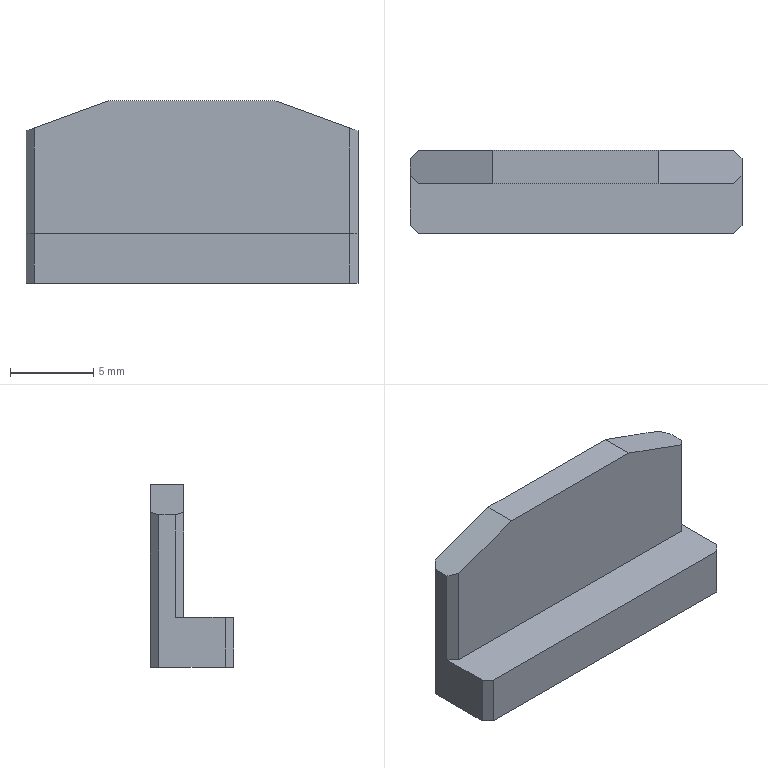Part | STEP file | QA-FB07 | 1 solid | 22 faces | box 20 x 5 x 11 mm | volume 541.763 mm3 | plane 18 | cylinder 4 | commonest cylinder face diameters 4.2 x4